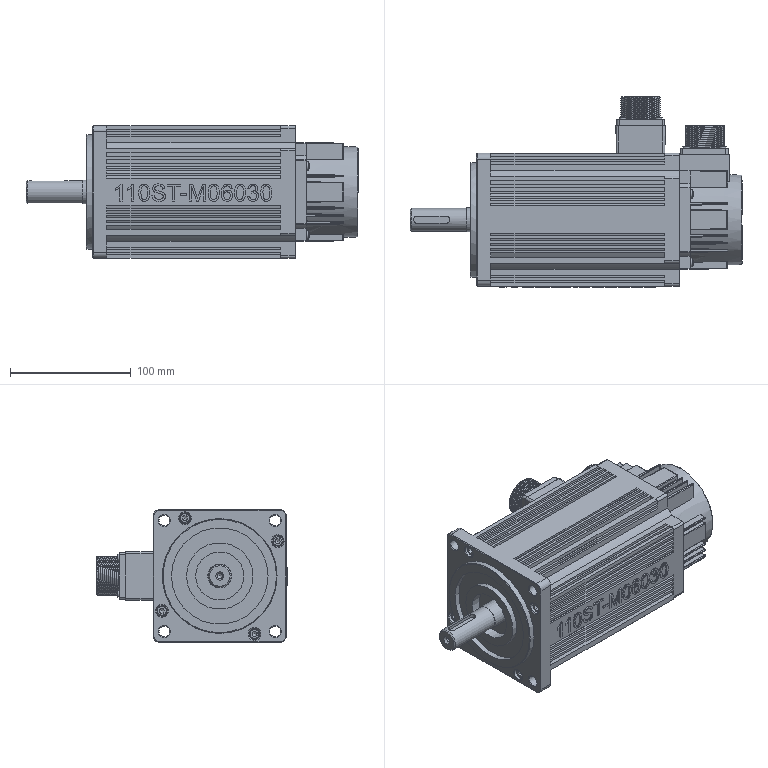Part | STEP file | YBQDJ-YB-22 | 25 solids | 1465 faces | box 275 x 158 x 110 mm | volume 3118501 mm3 | plane 854 | cylinder 371 | other 96 | cone 62 | sphere 44 | torus 31 | spline 7 | commonest cylinder face diameters 1 x107 0.6 x48 109 x32 4 x28 5 x12 5.5 x12